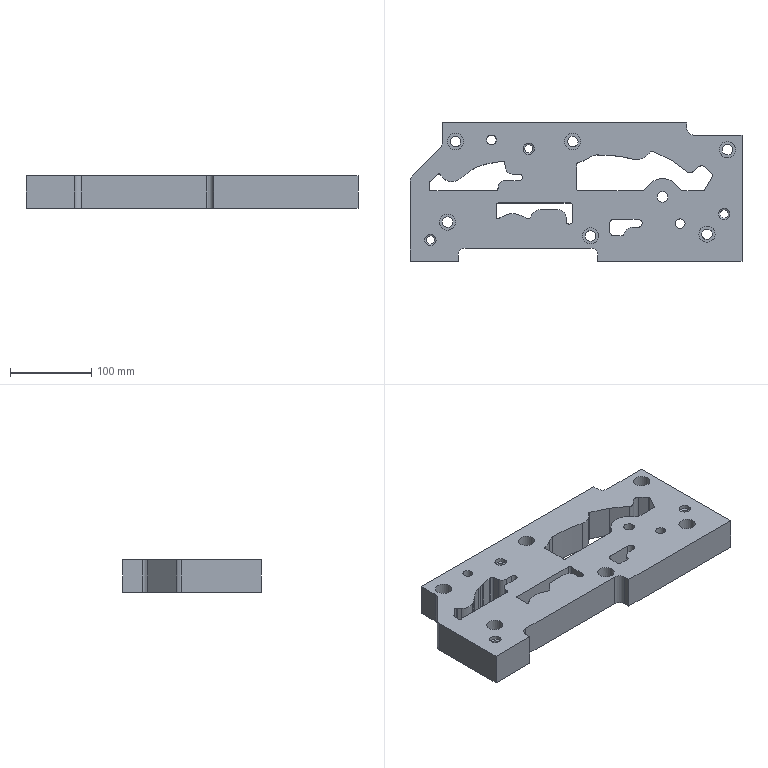Part | STEP file | gslz 2016.10.28-13_id182_x_t | 1 solid | 134 faces | box 408 x 170 x 40 mm | volume 2080328 mm3 | cylinder 71 | plane 60 | cone 3 | commonest cylinder face diameters 4 x16 20 x9 13 x7 10 x5 18 x5 16 x4